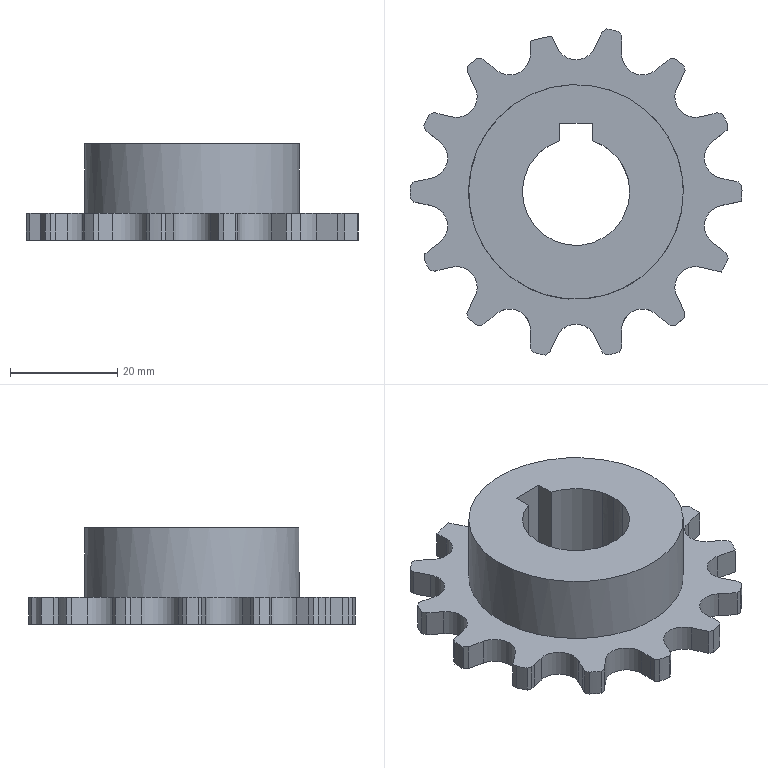Part | NX | features EXTRUDE 3, DATUM_CSYS 1, Delete Body 1, EXTRACT_DATUM_PLANE 1, SKETCH 1, UNITE 1 | 1 solid | 98 faces | box 61.9 x 60.843 x 18 mm | volume 22142 mm3 | plane 55 | cylinder 31 | spline 12 | commonest cylinder face diameters 7.77 x14 61.9 x13 20 x2 40 x1 58.797 x1